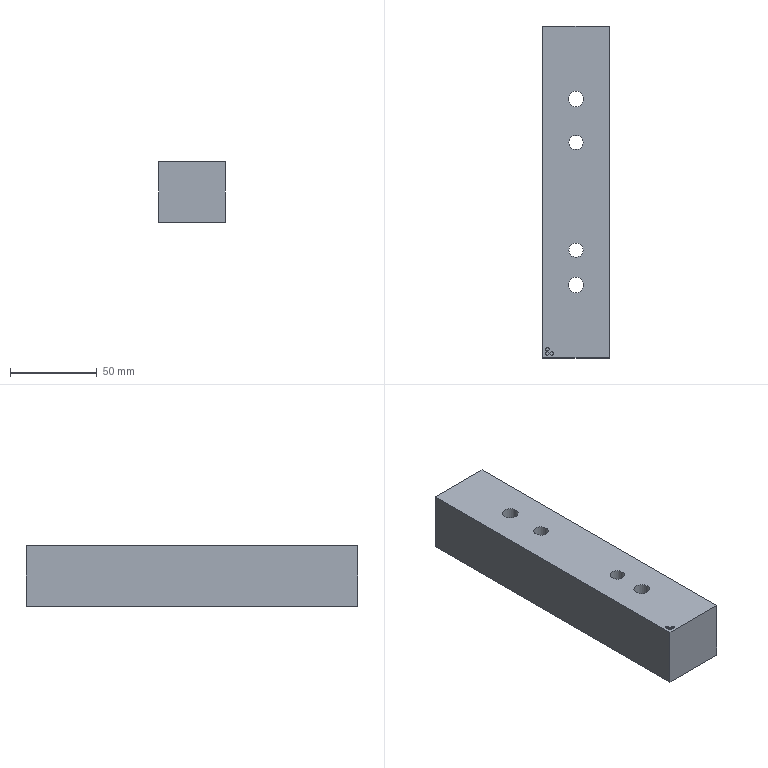Part | NX | features LB-1 2 | 1 solid | 16 faces | box 38 x 191 x 35 mm | volume 245823 mm3 | plane 9 | cylinder 7 | commonest cylinder face diameters 2 x3 8.25 x2 9.007 x2
STEP:
#1=CARTESIAN_POINT('',(2293.094,-763.622,803.716));
#2=VERTEX_POINT('',#1);
#3=CARTESIAN_POINT('',(2255.094,-763.622,803.716));
#4=VERTEX_POINT('',#3);
#5=CARTESIAN_POINT('',(2423.594,-763.622,803.716));
#6=DIRECTION('',(-1.,0.,0.));
#7=VECTOR('',#6,1000.);
#8=LINE('',#5,#7);
#9=EDGE_CURVE('',#2,#4,#8,.T.);
#10=ORIENTED_EDGE('',*,*,#9,.T.);
#11=CARTESIAN_POINT('',(2255.094,-763.622,838.716));
#12=VERTEX_POINT('',#11);
#13=CARTESIAN_POINT('',(2255.094,-763.622,838.716));
#14=DIRECTION('',(0.,0.,-1.));
#15=VECTOR('',#14,1000.);
#16=LINE('',#13,#15);
#17=EDGE_CURVE('',#12,#4,#16,.T.);
#18=ORIENTED_EDGE('',*,*,#17,.F.);
#19=CARTESIAN_POINT('',(2293.094,-763.622,838.716));
#20=VERTEX_POINT('',#19);
#21=CARTESIAN_POINT('',(2274.094,-763.622,838.716));
#22=DIRECTION('',(-1.,0.,0.));
#23=VECTOR('',#22,1000.);
#24=LINE('',#21,#23);
#25=EDGE_CURVE('',#20,#12,#24,.T.);
#26=ORIENTED_EDGE('',*,*,#25,.F.);
#27=CARTESIAN_POINT('',(2293.094,-763.622,838.716));
#28=DIRECTION('',(0.,0.,-1.));
#29=VECTOR('',#28,1000.);
#30=LINE('',#27,#29);
#31=EDGE_CURVE('',#20,#2,#30,.T.);
#32=ORIENTED_EDGE('',*,*,#31,.T.);
#33=EDGE_LOOP('',(#10,#18,#26,#32));
#34=FACE_BOUND('',#33,.T.);
#35=CARTESIAN_POINT('',(2293.094,-763.622,838.716));
#36=DIRECTION('',(0.,1.,0.));
#37=DIRECTION('',(0.,0.,-1.));
#38=AXIS2_PLACEMENT_3D('',#35,#36,#37);
#39=PLANE('',#38);
#40=ADVANCED_FACE('',(#34),#39,.T.);
#41=CARTESIAN_POINT('',(2255.094,-954.622,803.716));
#42=VERTEX_POINT('',#41);
#43=CARTESIAN_POINT('',(2255.094,-859.122,803.716));
#44=DIRECTION('',(0.,-1.,0.));
#45=VECTOR('',#44,1000.);
#46=LINE('',#43,#45);
#47=EDGE_CURVE('',#4,#42,#46,.T.);
#48=ORIENTED_EDGE('',*,*,#47,.T.);
#49=CARTESIAN_POINT('',(2255.094,-954.622,838.716));
#50=VERTEX_POINT('',#49);
#51=CARTESIAN_POINT('',(2255.094,-954.622,858.716));
#52=DIRECTION('',(0.,0.,-1.));
#53=VECTOR('',#52,1000.);
#54=LINE('',#51,#53);
#55=EDGE_CURVE('',#50,#42,#54,.T.);
#56=ORIENTED_EDGE('',*,*,#55,.F.);
#57=CARTESIAN_POINT('',(2255.094,-744.322,838.716));
#58=DIRECTION('',(0.,-1.,0.));
#59=VECTOR('',#58,1000.);
#60=LINE('',#57,#59);
#61=EDGE_CURVE('',#12,#50,#60,.T.);
#62=ORIENTED_EDGE('',*,*,#61,.F.);
#63=ORIENTED_EDGE('',*,*,#17,.T.);
#64=EDGE_LOOP('',(#48,#56,#62,#63));
#65=FACE_BOUND('',#64,.T.);
#66=CARTESIAN_POINT('',(2255.094,-744.322,838.716));
#67=DIRECTION('',(-1.,0.,0.));
#68=DIRECTION('',(0.,0.,-1.));
#69=AXIS2_PLACEMENT_3D('',#66,#67,#68);
#70=PLANE('',#69);
#71=ADVANCED_FACE('',(#65),#70,.T.);
#72=CARTESIAN_POINT('',(2293.094,-954.622,803.716));
#73=VERTEX_POINT('',#72);
#74=CARTESIAN_POINT('',(2423.594,-954.622,803.716));
#75=DIRECTION('',(1.,0.,0.));
#76=VECTOR('',#75,1000.);
#77=LINE('',#74,#76);
#78=EDGE_CURVE('',#42,#73,#77,.T.);
#79=ORIENTED_EDGE('',*,*,#78,.T.);
#80=CARTESIAN_POINT('',(2293.094,-954.622,838.716));
#81=VERTEX_POINT('',#80);
#82=CARTESIAN_POINT('',(2293.094,-954.622,838.716));
#83=DIRECTION('',(0.,0.,-1.));
#84=VECTOR('',#83,1000.);
#85=LINE('',#82,#84);
#86=EDGE_CURVE('',#81,#73,#85,.T.);
#87=ORIENTED_EDGE('',*,*,#86,.F.);
#88=CARTESIAN_POINT('',(2274.094,-954.622,838.716));
#89=DIRECTION('',(1.,0.,0.));
#90=VECTOR('',#89,1000.);
#91=LINE('',#88,#90);
#92=EDGE_CURVE('',#50,#81,#91,.T.);
#93=ORIENTED_EDGE('',*,*,#92,.F.);
#94=ORIENTED_EDGE('',*,*,#55,.T.);
#95=EDGE_LOOP('',(#79,#87,#93,#94));
#96=FACE_BOUND('',#95,.T.);
#97=CARTESIAN_POINT('',(2118.094,-954.622,858.716));
#98=DIRECTION('',(0.,-1.,0.));
#99=DIRECTION('',(0.,0.,1.));
#100=AXIS2_PLACEMENT_3D('',#97,#98,#99);
#101=PLANE('',#100);
#102=ADVANCED_FACE('',(#96),#101,.T.);
#103=CARTESIAN_POINT('',(2293.094,-859.122,803.716));
#104=DIRECTION('',(0.,1.,0.));
#105=VECTOR('',#104,1000.);
#106=LINE('',#103,#105);
#107=EDGE_CURVE('',#73,#2,#106,.T.);
#108=ORIENTED_EDGE('',*,*,#107,.T.);
#109=ORIENTED_EDGE('',*,*,#31,.F.);
#110=CARTESIAN_POINT('',(2293.094,-917.322,838.716));
#111=DIRECTION('',(0.,1.,0.));
#112=VECTOR('',#111,1000.);
#113=LINE('',#110,#112);
#114=EDGE_CURVE('',#81,#20,#113,.T.);
#115=ORIENTED_EDGE('',*,*,#114,.F.);
#116=ORIENTED_EDGE('',*,*,#86,.T.);
#117=EDGE_LOOP('',(#108,#109,#115,#116));
#118=FACE_BOUND('',#117,.T.);
#119=CARTESIAN_POINT('',(2293.094,-917.322,838.716));
#120=DIRECTION('',(1.,0.,0.));
#121=DIRECTION('',(0.,0.,1.));
#122=AXIS2_PLACEMENT_3D('',#119,#120,#121);
#123=PLANE('',#122);
#124=ADVANCED_FACE('',(#118),#123,.T.);
#125=CARTESIAN_POINT('',(2269.59,-912.622,803.716));
#126=VERTEX_POINT('',#125);
#127=CARTESIAN_POINT('',(2274.094,-912.622,803.716));
#128=DIRECTION('',(0.,0.,-1.));
#129=DIRECTION('',(-1.,0.,0.));
#130=AXIS2_PLACEMENT_3D('',#127,#128,#129);
#131=CIRCLE('',#130,4.503);
#132=EDGE_CURVE('',#126,#126,#131,.T.);
#133=ORIENTED_EDGE('',*,*,#132,.F.);
#134=EDGE_LOOP('',(#133));
#135=FACE_BOUND('',#134,.T.);
#136=CARTESIAN_POINT('',(2269.59,-805.622,803.716));
#137=VERTEX_POINT('',#136);
#138=CARTESIAN_POINT('',(2274.094,-805.622,803.716));
#139=DIRECTION('',(0.,0.,-1.));
#140=DIRECTION('',(-1.,0.,0.));
#141=AXIS2_PLACEMENT_3D('',#138,#139,#140);
#142=CIRCLE('',#141,4.503);
#143=EDGE_CURVE('',#137,#137,#142,.T.);
#144=ORIENTED_EDGE('',*,*,#143,.F.);
#145=EDGE_LOOP('',(#144));
#146=FACE_BOUND('',#145,.T.);
#147=CARTESIAN_POINT('',(2269.969,-892.622,803.716));
#148=VERTEX_POINT('',#147);
#149=CARTESIAN_POINT('',(2274.094,-892.622,803.716));
#150=DIRECTION('',(0.,0.,-1.));
#151=DIRECTION('',(-1.,0.,0.));
#152=AXIS2_PLACEMENT_3D('',#149,#150,#151);
#153=CIRCLE('',#152,4.125);
#154=EDGE_CURVE('',#148,#148,#153,.T.);
#155=ORIENTED_EDGE('',*,*,#154,.F.);
#156=EDGE_LOOP('',(#155));
#157=FACE_BOUND('',#156,.T.);
#158=CARTESIAN_POINT('',(2269.969,-830.622,803.716));
#159=VERTEX_POINT('',#158);
#160=CARTESIAN_POINT('',(2274.094,-830.622,803.716));
#161=DIRECTION('',(0.,0.,-1.));
#162=DIRECTION('',(-1.,0.,0.));
#163=AXIS2_PLACEMENT_3D('',#160,#161,#162);
#164=CIRCLE('',#163,4.125);
#165=EDGE_CURVE('',#159,#159,#164,.T.);
#166=ORIENTED_EDGE('',*,*,#165,.F.);
#167=EDGE_LOOP('',(#166));
#168=FACE_BOUND('',#167,.T.);
#169=ORIENTED_EDGE('',*,*,#9,.F.);
#170=ORIENTED_EDGE('',*,*,#107,.F.);
#171=ORIENTED_EDGE('',*,*,#78,.F.);
#172=ORIENTED_EDGE('',*,*,#47,.F.);
#173=EDGE_LOOP('',(#169,#170,#171,#172));
#174=FACE_BOUND('',#173,.T.);
#175=CARTESIAN_POINT('',(2423.594,-859.122,803.716));
#176=DIRECTION('',(0.,0.,-1.));
#177=DIRECTION('',(1.,0.,0.));
#178=AXIS2_PLACEMENT_3D('',#175,#176,#177);
#179=PLANE('',#178);
#180=ADVANCED_FACE('',(#135,#146,#157,#168,#174),#179,.T.);
#181=CARTESIAN_POINT('',(2258.594,-949.622,838.716));
#182=VERTEX_POINT('',#181);
#183=CARTESIAN_POINT('',(2257.594,-949.622,838.716));
#184=DIRECTION('',(0.,0.,1.));
#185=DIRECTION('',(1.,0.,0.));
#186=AXIS2_PLACEMENT_3D('',#183,#184,#185);
#187=CIRCLE('',#186,1.);
#188=EDGE_CURVE('',#182,#182,#187,.T.);
#189=ORIENTED_EDGE('',*,*,#188,.F.);
#190=EDGE_LOOP('',(#189));
#191=FACE_BOUND('',#190,.T.);
#192=CARTESIAN_POINT('',(2261.094,-952.122,838.716));
#193=VERTEX_POINT('',#192);
#194=CARTESIAN_POINT('',(2260.094,-952.122,838.716));
#195=DIRECTION('',(0.,0.,1.));
#196=DIRECTION('',(1.,0.,0.));
#197=AXIS2_PLACEMENT_3D('',#194,#195,#196);
#198=CIRCLE('',#197,1.);
#199=EDGE_CURVE('',#193,#193,#198,.T.);
#200=ORIENTED_EDGE('',*,*,#199,.F.);
#201=EDGE_LOOP('',(#200));
#202=FACE_BOUND('',#201,.T.);
#203=CARTESIAN_POINT('',(2258.594,-952.122,838.716));
#204=VERTEX_POINT('',#203);
#205=CARTESIAN_POINT('',(2257.594,-952.122,838.716));
#206=DIRECTION('',(0.,0.,1.));
#207=DIRECTION('',(1.,0.,0.));
#208=AXIS2_PLACEMENT_3D('',#205,#206,#207);
#209=CIRCLE('',#208,1.);
#210=EDGE_CURVE('',#204,#204,#209,.T.);
#211=ORIENTED_EDGE('',*,*,#210,.F.);
#212=EDGE_LOOP('',(#211));
#213=FACE_BOUND('',#212,.T.);
#214=CARTESIAN_POINT('',(2278.597,-912.622,838.716));
#215=VERTEX_POINT('',#214);
#216=CARTESIAN_POINT('',(2274.094,-912.622,838.716));
#217=DIRECTION('',(0.,0.,1.));
#218=DIRECTION('',(1.,0.,0.));
#219=AXIS2_PLACEMENT_3D('',#216,#217,#218);
#220=CIRCLE('',#219,4.503);
#221=EDGE_CURVE('',#215,#215,#220,.F.);
#222=ORIENTED_EDGE('',*,*,#221,.T.);
#223=EDGE_LOOP('',(#222));
#224=FACE_BOUND('',#223,.T.);
#225=CARTESIAN_POINT('',(2278.597,-805.622,838.716));
#226=VERTEX_POINT('',#225);
#227=CARTESIAN_POINT('',(2274.094,-805.622,838.716));
#228=DIRECTION('',(0.,0.,1.));
#229=DIRECTION('',(1.,0.,0.));
#230=AXIS2_PLACEMENT_3D('',#227,#228,#229);
#231=CIRCLE('',#230,4.503);
#232=EDGE_CURVE('',#226,#226,#231,.F.);
#233=ORIENTED_EDGE('',*,*,#232,.T.);
#234=EDGE_LOOP('',(#233));
#235=FACE_BOUND('',#234,.T.);
#236=CARTESIAN_POINT('',(2278.219,-892.622,838.716));
#237=VERTEX_POINT('',#236);
#238=CARTESIAN_POINT('',(2274.094,-892.622,838.716));
#239=DIRECTION('',(0.,0.,-1.));
#240=DIRECTION('',(1.,0.,0.));
#241=AXIS2_PLACEMENT_3D('',#238,#239,#240);
#242=CIRCLE('',#241,4.125);
#243=EDGE_CURVE('',#237,#237,#242,.T.);
#244=ORIENTED_EDGE('',*,*,#243,.T.);
#245=EDGE_LOOP('',(#244));
#246=FACE_BOUND('',#245,.T.);
#247=CARTESIAN_POINT('',(2278.219,-830.622,838.716));
#248=VERTEX_POINT('',#247);
#249=CARTESIAN_POINT('',(2274.094,-830.622,838.716));
#250=DIRECTION('',(0.,0.,-1.));
#251=DIRECTION('',(1.,0.,0.));
#252=AXIS2_PLACEMENT_3D('',#249,#250,#251);
#253=CIRCLE('',#252,4.125);
#254=EDGE_CURVE('',#248,#248,#253,.T.);
#255=ORIENTED_EDGE('',*,*,#254,.T.);
#256=EDGE_LOOP('',(#255));
#257=FACE_BOUND('',#256,.T.);
#258=ORIENTED_EDGE('',*,*,#114,.T.);
#259=ORIENTED_EDGE('',*,*,#25,.T.);
#260=ORIENTED_EDGE('',*,*,#61,.T.);
#261=ORIENTED_EDGE('',*,*,#92,.T.);
#262=EDGE_LOOP('',(#258,#259,#260,#261));
#263=FACE_BOUND('',#262,.T.);
#264=CARTESIAN_POINT('',(2274.094,-830.822,838.716));
#265=DIRECTION('',(0.,0.,1.));
#266=DIRECTION('',(-1.,0.,0.));
#267=AXIS2_PLACEMENT_3D('',#264,#265,#266);
#268=PLANE('',#267);
#269=ADVANCED_FACE('',(#191,#202,#213,#224,#235,#246,#257,#263),#268,.T.);
#270=ORIENTED_EDGE('',*,*,#165,.T.);
#271=EDGE_LOOP('',(#270));
#272=FACE_BOUND('',#271,.T.);
#273=ORIENTED_EDGE('',*,*,#254,.F.);
#274=EDGE_LOOP('',(#273));
#275=FACE_BOUND('',#274,.T.);
#276=CARTESIAN_POINT('',(2274.094,-830.622,838.716));
#277=DIRECTION('',(0.,0.,-1.));
#278=DIRECTION('',(1.,0.,0.));
#279=AXIS2_PLACEMENT_3D('',#276,#277,#278);
#280=CYLINDRICAL_SURFACE('',#279,4.125);
#281=ADVANCED_FACE('',(#272,#275),#280,.F.);
#282=ORIENTED_EDGE('',*,*,#154,.T.);
#283=EDGE_LOOP('',(#282));
#284=FACE_BOUND('',#283,.T.);
#285=ORIENTED_EDGE('',*,*,#243,.F.);
#286=EDGE_LOOP('',(#285));
#287=FACE_BOUND('',#286,.T.);
#288=CARTESIAN_POINT('',(2274.094,-892.622,838.716));
#289=DIRECTION('',(0.,0.,-1.));
#290=DIRECTION('',(1.,0.,0.));
#291=AXIS2_PLACEMENT_3D('',#288,#289,#290);
#292=CYLINDRICAL_SURFACE('',#291,4.125);
#293=ADVANCED_FACE('',(#284,#287),#292,.F.);
#294=ORIENTED_EDGE('',*,*,#143,.T.);
#295=EDGE_LOOP('',(#294));
#296=FACE_BOUND('',#295,.T.);
#297=ORIENTED_EDGE('',*,*,#232,.F.);
#298=EDGE_LOOP('',(#297));
#299=FACE_BOUND('',#298,.T.);
#300=CARTESIAN_POINT('',(2274.094,-805.622,838.716));
#301=DIRECTION('',(0.,0.,-1.));
#302=DIRECTION('',(1.,0.,0.));
#303=AXIS2_PLACEMENT_3D('',#300,#301,#302);
#304=CYLINDRICAL_SURFACE('',#303,4.503);
#305=ADVANCED_FACE('',(#296,#299),#304,.F.);
#306=ORIENTED_EDGE('',*,*,#132,.T.);
#307=EDGE_LOOP('',(#306));
#308=FACE_BOUND('',#307,.T.);
#309=ORIENTED_EDGE('',*,*,#221,.F.);
#310=EDGE_LOOP('',(#309));
#311=FACE_BOUND('',#310,.T.);
#312=CARTESIAN_POINT('',(2274.094,-912.622,838.716));
#313=DIRECTION('',(0.,0.,-1.));
#314=DIRECTION('',(1.,0.,0.));
#315=AXIS2_PLACEMENT_3D('',#312,#313,#314);
#316=CYLINDRICAL_SURFACE('',#315,4.503);
#317=ADVANCED_FACE('',(#308,#311),#316,.F.);
#318=CARTESIAN_POINT('',(2258.594,-952.122,838.216));
#319=VERTEX_POINT('',#318);
#320=CARTESIAN_POINT('',(2257.594,-952.122,838.216));
#321=DIRECTION('',(0.,0.,1.));
#322=DIRECTION('',(1.,0.,0.));
#323=AXIS2_PLACEMENT_3D('',#320,#321,#322);
#324=CIRCLE('',#323,1.);
#325=EDGE_CURVE('',#319,#319,#324,.F.);
#326=ORIENTED_EDGE('',*,*,#325,.T.);
#327=EDGE_LOOP('',(#326));
#328=FACE_BOUND('',#327,.T.);
#329=ORIENTED_EDGE('',*,*,#210,.T.);
#330=EDGE_LOOP('',(#329));
#331=FACE_BOUND('',#330,.T.);
#332=CARTESIAN_POINT('',(2257.594,-952.122,838.216));
#333=DIRECTION('',(0.,0.,1.));
#334=DIRECTION('',(1.,0.,0.));
#335=AXIS2_PLACEMENT_3D('',#332,#333,#334);
#336=CYLINDRICAL_SURFACE('',#335,1.);
#337=ADVANCED_FACE('',(#328,#331),#336,.F.);
#338=ORIENTED_EDGE('',*,*,#325,.F.);
#339=EDGE_LOOP('',(#338));
#340=FACE_BOUND('',#339,.T.);
#341=CARTESIAN_POINT('',(2257.594,-952.122,838.216));
#342=DIRECTION('',(0.,0.,1.));
#343=DIRECTION('',(1.,0.,0.));
#344=AXIS2_PLACEMENT_3D('',#341,#342,#343);
#345=PLANE('',#344);
#346=ADVANCED_FACE('',(#340),#345,.T.);
#347=CARTESIAN_POINT('',(2261.094,-952.122,838.216));
#348=VERTEX_POINT('',#347);
#349=CARTESIAN_POINT('',(2260.094,-952.122,838.216));
#350=DIRECTION('',(0.,0.,1.));
#351=DIRECTION('',(1.,0.,0.));
#352=AXIS2_PLACEMENT_3D('',#349,#350,#351);
#353=CIRCLE('',#352,1.);
#354=EDGE_CURVE('',#348,#348,#353,.F.);
#355=ORIENTED_EDGE('',*,*,#354,.T.);
#356=EDGE_LOOP('',(#355));
#357=FACE_BOUND('',#356,.T.);
#358=ORIENTED_EDGE('',*,*,#199,.T.);
#359=EDGE_LOOP('',(#358));
#360=FACE_BOUND('',#359,.T.);
#361=CARTESIAN_POINT('',(2260.094,-952.122,838.216));
#362=DIRECTION('',(0.,0.,1.));
#363=DIRECTION('',(1.,0.,0.));
#364=AXIS2_PLACEMENT_3D('',#361,#362,#363);
#365=CYLINDRICAL_SURFACE('',#364,1.);
#366=ADVANCED_FACE('',(#357,#360),#365,.F.);
#367=ORIENTED_EDGE('',*,*,#354,.F.);
#368=EDGE_LOOP('',(#367));
#369=FACE_BOUND('',#368,.T.);
#370=CARTESIAN_POINT('',(2260.094,-952.122,838.216));
#371=DIRECTION('',(0.,0.,1.));
#372=DIRECTION('',(1.,0.,0.));
#373=AXIS2_PLACEMENT_3D('',#370,#371,#372);
#374=PLANE('',#373);
#375=ADVANCED_FACE('',(#369),#374,.T.);
#376=CARTESIAN_POINT('',(2258.594,-949.622,838.216));
#377=VERTEX_POINT('',#376);
#378=CARTESIAN_POINT('',(2257.594,-949.622,838.216));
#379=DIRECTION('',(0.,0.,1.));
#380=DIRECTION('',(1.,0.,0.));
#381=AXIS2_PLACEMENT_3D('',#378,#379,#380);
#382=CIRCLE('',#381,1.);
#383=EDGE_CURVE('',#377,#377,#382,.F.);
#384=ORIENTED_EDGE('',*,*,#383,.T.);
#385=EDGE_LOOP('',(#384));
#386=FACE_BOUND('',#385,.T.);
#387=ORIENTED_EDGE('',*,*,#188,.T.);
#388=EDGE_LOOP('',(#387));
#389=FACE_BOUND('',#388,.T.);
#390=CARTESIAN_POINT('',(2257.594,-949.622,838.216));
#391=DIRECTION('',(0.,0.,1.));
#392=DIRECTION('',(1.,0.,0.));
#393=AXIS2_PLACEMENT_3D('',#390,#391,#392);
#394=CYLINDRICAL_SURFACE('',#393,1.);
#395=ADVANCED_FACE('',(#386,#389),#394,.F.);
#396=ORIENTED_EDGE('',*,*,#383,.F.);
#397=EDGE_LOOP('',(#396));
#398=FACE_BOUND('',#397,.T.);
#399=CARTESIAN_POINT('',(2257.594,-949.622,838.216));
#400=DIRECTION('',(0.,0.,1.));
#401=DIRECTION('',(1.,0.,0.));
#402=AXIS2_PLACEMENT_3D('',#399,#400,#401);
#403=PLANE('',#402);
#404=ADVANCED_FACE('',(#398),#403,.T.);
#405=CLOSED_SHELL('',(#40,#71,#102,#124,#180,#269,#281,#293,#305,#317,#337,#346,#366,#375,#395,#404));
#406=MANIFOLD_SOLID_BREP('',#405);
#407=(LENGTH_UNIT()NAMED_UNIT(*)SI_UNIT(.MILLI.,.METRE.));
#408=UNCERTAINTY_MEASURE_WITH_UNIT(LENGTH_MEASURE(0.00001),#407,'','');
#409=(NAMED_UNIT(*)PLANE_ANGLE_UNIT()SI_UNIT($,.RADIAN.));
#410=(NAMED_UNIT(*)SI_UNIT($,.STERADIAN.)SOLID_ANGLE_UNIT());
#411=(GEOMETRIC_REPRESENTATION_CONTEXT(3)GLOBAL_UNCERTAINTY_ASSIGNED_CONTEXT((#408))GLOBAL_UNIT_ASSIGNED_CONTEXT((#407,#409,#410))REPRESENTATION_CONTEXT('',''));
#412=ADVANCED_BREP_SHAPE_REPRESENTATION('',(#406),#411);